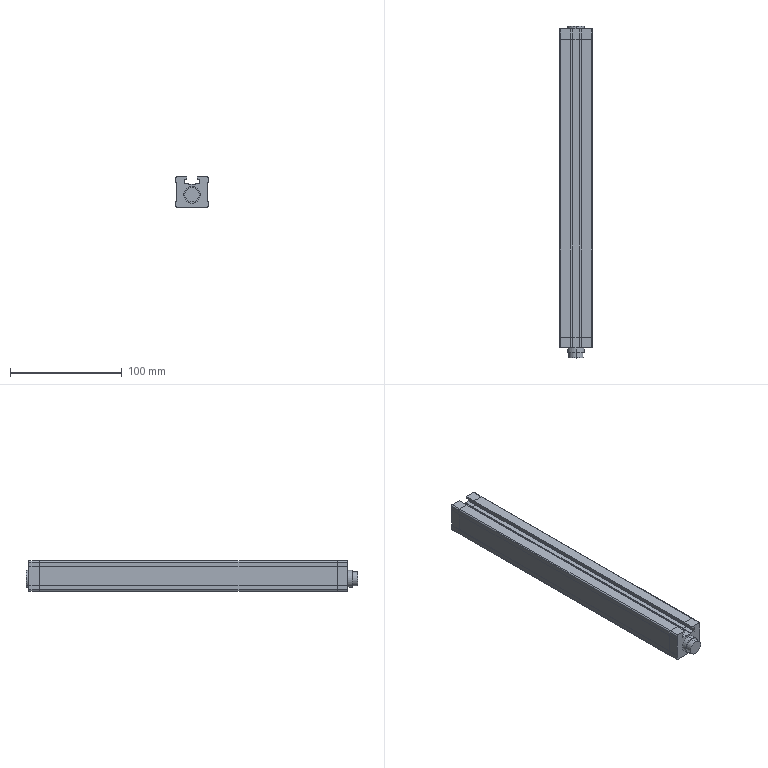Part | STEP file | STD-NB1220 safety light curtain | 1 solid | 103 faces | box 29 x 296.5 x 27 mm | volume 192265 mm3 | plane 85 | cylinder 18 | commonest cylinder face diameters 1.96 x8 2 x4 15 x4 12.7 x2